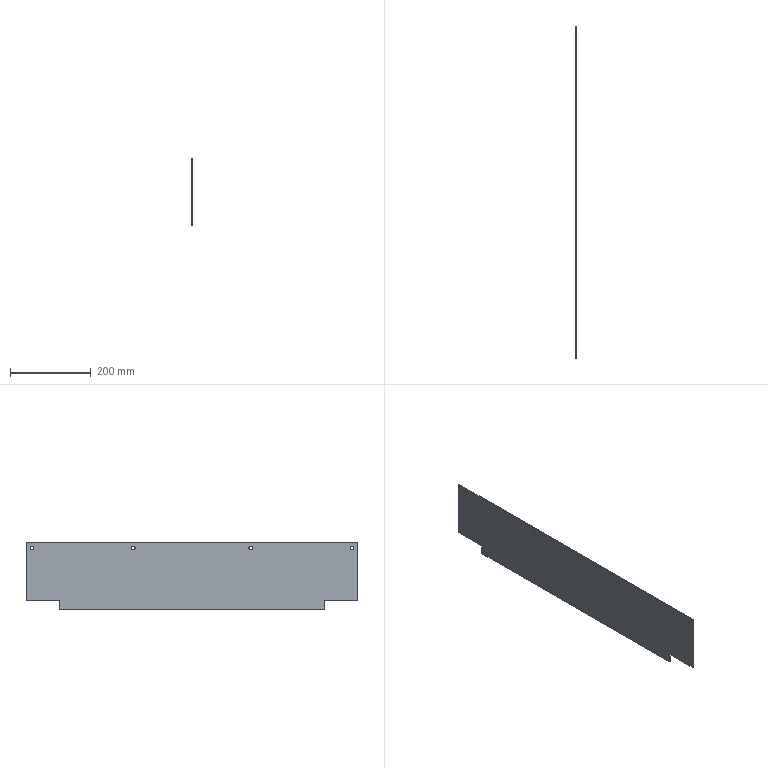Part | STEP file | lll_id2674_x_t | 1 solid | 14 faces | box 2 x 820 x 168 mm | volume 267265 mm3 | plane 10 | cylinder 4 | commonest cylinder face diameters 9 x4
STEP:
#1=CARTESIAN_POINT('',(165.435,-327.7,2.5));
#2=VERTEX_POINT('',#1);
#3=CARTESIAN_POINT('',(165.435,327.5,2.5));
#4=VERTEX_POINT('',#3);
#5=CARTESIAN_POINT('',(165.435,60.,2.5));
#6=DIRECTION('',(0.,1.,0.));
#7=VECTOR('',#6,1.);
#8=LINE('',#5,#7);
#9=EDGE_CURVE('',#2,#4,#8,.T.);
#10=ORIENTED_EDGE('',*,*,#9,.T.);
#11=CARTESIAN_POINT('',(167.435,327.5,2.5));
#12=VERTEX_POINT('',#11);
#13=CARTESIAN_POINT('',(651.435,327.5,2.5));
#14=DIRECTION('',(1.,0.,0.));
#15=VECTOR('',#14,1.);
#16=LINE('',#13,#15);
#17=EDGE_CURVE('',#4,#12,#16,.T.);
#18=ORIENTED_EDGE('',*,*,#17,.T.);
#19=CARTESIAN_POINT('',(167.435,-327.7,2.5));
#20=VERTEX_POINT('',#19);
#21=CARTESIAN_POINT('',(167.435,60.,2.5));
#22=DIRECTION('',(0.,1.,0.));
#23=VECTOR('',#22,1.);
#24=LINE('',#21,#23);
#25=EDGE_CURVE('',#20,#12,#24,.T.);
#26=ORIENTED_EDGE('',*,*,#25,.F.);
#27=CARTESIAN_POINT('',(651.435,-327.7,2.5));
#28=DIRECTION('',(-1.,0.,0.));
#29=VECTOR('',#28,1.);
#30=LINE('',#27,#29);
#31=EDGE_CURVE('',#20,#2,#30,.T.);
#32=ORIENTED_EDGE('',*,*,#31,.T.);
#33=EDGE_LOOP('',(#10,#18,#26,#32));
#34=FACE_OUTER_BOUND('',#33,.T.);
#35=CARTESIAN_POINT('',(651.435,1252.5,2.5));
#36=DIRECTION('',(0.,0.,-1.));
#37=DIRECTION('',(0.,-1.,0.));
#38=AXIS2_PLACEMENT_3D('',#35,#36,#37);
#39=PLANE('',#38);
#40=ADVANCED_FACE('',(#34),#39,.T.);
#41=CARTESIAN_POINT('',(165.435,140.5,155.5));
#42=VERTEX_POINT('',#41);
#43=CARTESIAN_POINT('',(165.435,145.,155.5));
#44=DIRECTION('',(1.,0.,0.));
#45=DIRECTION('',(0.,-1.,0.));
#46=AXIS2_PLACEMENT_3D('',#43,#44,#45);
#47=CIRCLE('',#46,4.5);
#48=EDGE_CURVE('',#42,#42,#47,.T.);
#49=ORIENTED_EDGE('',*,*,#48,.T.);
#50=EDGE_LOOP('',(#49));
#51=FACE_BOUND('',#50,.T.);
#52=CARTESIAN_POINT('',(165.435,399.5,155.5));
#53=VERTEX_POINT('',#52);
#54=CARTESIAN_POINT('',(165.435,395.,155.5));
#55=DIRECTION('',(1.,0.,0.));
#56=DIRECTION('',(0.,1.,0.));
#57=AXIS2_PLACEMENT_3D('',#54,#55,#56);
#58=CIRCLE('',#57,4.5);
#59=EDGE_CURVE('',#53,#53,#58,.T.);
#60=ORIENTED_EDGE('',*,*,#59,.T.);
#61=EDGE_LOOP('',(#60));
#62=FACE_BOUND('',#61,.T.);
#63=CARTESIAN_POINT('',(165.435,-140.5,155.5));
#64=VERTEX_POINT('',#63);
#65=CARTESIAN_POINT('',(165.435,-145.,155.5));
#66=DIRECTION('',(-1.,0.,0.));
#67=DIRECTION('',(0.,1.,0.));
#68=AXIS2_PLACEMENT_3D('',#65,#66,#67);
#69=CIRCLE('',#68,4.5);
#70=EDGE_CURVE('',#64,#64,#69,.T.);
#71=ORIENTED_EDGE('',*,*,#70,.F.);
#72=EDGE_LOOP('',(#71));
#73=FACE_BOUND('',#72,.T.);
#74=CARTESIAN_POINT('',(165.435,-399.5,155.5));
#75=VERTEX_POINT('',#74);
#76=CARTESIAN_POINT('',(165.435,-395.,155.5));
#77=DIRECTION('',(-1.,0.,0.));
#78=DIRECTION('',(0.,-1.,0.));
#79=AXIS2_PLACEMENT_3D('',#76,#77,#78);
#80=CIRCLE('',#79,4.5);
#81=EDGE_CURVE('',#75,#75,#80,.T.);
#82=ORIENTED_EDGE('',*,*,#81,.F.);
#83=EDGE_LOOP('',(#82));
#84=FACE_BOUND('',#83,.T.);
#85=CARTESIAN_POINT('',(165.435,327.5,26.));
#86=VERTEX_POINT('',#85);
#87=CARTESIAN_POINT('',(165.435,327.5,-78.5));
#88=DIRECTION('',(0.,0.,1.));
#89=VECTOR('',#88,1.);
#90=LINE('',#87,#89);
#91=EDGE_CURVE('',#4,#86,#90,.T.);
#92=ORIENTED_EDGE('',*,*,#91,.F.);
#93=ORIENTED_EDGE('',*,*,#9,.F.);
#94=CARTESIAN_POINT('',(165.435,-327.7,26.));
#95=VERTEX_POINT('',#94);
#96=CARTESIAN_POINT('',(165.435,-327.7,-78.5));
#97=DIRECTION('',(0.,0.,-1.));
#98=VECTOR('',#97,1.);
#99=LINE('',#96,#98);
#100=EDGE_CURVE('',#95,#2,#99,.T.);
#101=ORIENTED_EDGE('',*,*,#100,.F.);
#102=CARTESIAN_POINT('',(165.435,-410.,26.));
#103=VERTEX_POINT('',#102);
#104=CARTESIAN_POINT('',(165.435,60.,26.));
#105=DIRECTION('',(0.,1.,0.));
#106=VECTOR('',#105,1.);
#107=LINE('',#104,#106);
#108=EDGE_CURVE('',#103,#95,#107,.T.);
#109=ORIENTED_EDGE('',*,*,#108,.F.);
#110=CARTESIAN_POINT('',(165.435,-410.,170.5));
#111=VERTEX_POINT('',#110);
#112=CARTESIAN_POINT('',(165.435,-410.,-78.5));
#113=DIRECTION('',(0.,0.,-1.));
#114=VECTOR('',#113,1.);
#115=LINE('',#112,#114);
#116=EDGE_CURVE('',#111,#103,#115,.T.);
#117=ORIENTED_EDGE('',*,*,#116,.F.);
#118=CARTESIAN_POINT('',(165.435,410.,170.5));
#119=VERTEX_POINT('',#118);
#120=CARTESIAN_POINT('',(165.435,60.,170.5));
#121=DIRECTION('',(0.,-1.,0.));
#122=VECTOR('',#121,1.);
#123=LINE('',#120,#122);
#124=EDGE_CURVE('',#119,#111,#123,.T.);
#125=ORIENTED_EDGE('',*,*,#124,.F.);
#126=CARTESIAN_POINT('',(165.435,410.,26.));
#127=VERTEX_POINT('',#126);
#128=CARTESIAN_POINT('',(165.435,410.,-78.5));
#129=DIRECTION('',(0.,0.,-1.));
#130=VECTOR('',#129,1.);
#131=LINE('',#128,#130);
#132=EDGE_CURVE('',#119,#127,#131,.T.);
#133=ORIENTED_EDGE('',*,*,#132,.T.);
#134=CARTESIAN_POINT('',(165.435,60.,26.));
#135=DIRECTION('',(0.,1.,0.));
#136=VECTOR('',#135,1.);
#137=LINE('',#134,#136);
#138=EDGE_CURVE('',#86,#127,#137,.T.);
#139=ORIENTED_EDGE('',*,*,#138,.F.);
#140=EDGE_LOOP('',(#92,#93,#101,#109,#117,#125,#133,#139));
#141=FACE_BOUND('',#140,.T.);
#142=CARTESIAN_POINT('',(165.435,60.,-78.5));
#143=DIRECTION('',(1.,0.,0.));
#144=DIRECTION('',(0.,0.,-1.));
#145=AXIS2_PLACEMENT_3D('',#142,#143,#144);
#146=PLANE('',#145);
#147=ADVANCED_FACE('',(#51,#62,#73,#84,#141),#146,.F.);
#148=CARTESIAN_POINT('',(167.435,-390.5,155.5));
#149=VERTEX_POINT('',#148);
#150=CARTESIAN_POINT('',(167.435,-395.,155.5));
#151=DIRECTION('',(-1.,0.,0.));
#152=DIRECTION('',(0.,1.,0.));
#153=AXIS2_PLACEMENT_3D('',#150,#151,#152);
#154=CIRCLE('',#153,4.5);
#155=EDGE_CURVE('',#149,#149,#154,.T.);
#156=ORIENTED_EDGE('',*,*,#155,.T.);
#157=EDGE_LOOP('',(#156));
#158=FACE_BOUND('',#157,.T.);
#159=CARTESIAN_POINT('',(167.435,-140.5,155.5));
#160=VERTEX_POINT('',#159);
#161=CARTESIAN_POINT('',(167.435,-145.,155.5));
#162=DIRECTION('',(-1.,0.,0.));
#163=DIRECTION('',(0.,1.,0.));
#164=AXIS2_PLACEMENT_3D('',#161,#162,#163);
#165=CIRCLE('',#164,4.5);
#166=EDGE_CURVE('',#160,#160,#165,.T.);
#167=ORIENTED_EDGE('',*,*,#166,.T.);
#168=EDGE_LOOP('',(#167));
#169=FACE_BOUND('',#168,.T.);
#170=CARTESIAN_POINT('',(167.435,390.5,155.5));
#171=VERTEX_POINT('',#170);
#172=CARTESIAN_POINT('',(167.435,395.,155.5));
#173=DIRECTION('',(1.,0.,0.));
#174=DIRECTION('',(0.,-1.,0.));
#175=AXIS2_PLACEMENT_3D('',#172,#173,#174);
#176=CIRCLE('',#175,4.5);
#177=EDGE_CURVE('',#171,#171,#176,.T.);
#178=ORIENTED_EDGE('',*,*,#177,.F.);
#179=EDGE_LOOP('',(#178));
#180=FACE_BOUND('',#179,.T.);
#181=CARTESIAN_POINT('',(167.435,140.5,155.5));
#182=VERTEX_POINT('',#181);
#183=CARTESIAN_POINT('',(167.435,145.,155.5));
#184=DIRECTION('',(1.,0.,0.));
#185=DIRECTION('',(0.,-1.,0.));
#186=AXIS2_PLACEMENT_3D('',#183,#184,#185);
#187=CIRCLE('',#186,4.5);
#188=EDGE_CURVE('',#182,#182,#187,.T.);
#189=ORIENTED_EDGE('',*,*,#188,.F.);
#190=EDGE_LOOP('',(#189));
#191=FACE_BOUND('',#190,.T.);
#192=ORIENTED_EDGE('',*,*,#25,.T.);
#193=CARTESIAN_POINT('',(167.435,327.5,26.));
#194=VERTEX_POINT('',#193);
#195=CARTESIAN_POINT('',(167.435,327.5,-78.5));
#196=DIRECTION('',(0.,0.,1.));
#197=VECTOR('',#196,1.);
#198=LINE('',#195,#197);
#199=EDGE_CURVE('',#12,#194,#198,.T.);
#200=ORIENTED_EDGE('',*,*,#199,.T.);
#201=CARTESIAN_POINT('',(167.435,410.,26.));
#202=VERTEX_POINT('',#201);
#203=CARTESIAN_POINT('',(167.435,60.,26.));
#204=DIRECTION('',(0.,1.,0.));
#205=VECTOR('',#204,1.);
#206=LINE('',#203,#205);
#207=EDGE_CURVE('',#194,#202,#206,.T.);
#208=ORIENTED_EDGE('',*,*,#207,.T.);
#209=CARTESIAN_POINT('',(167.435,410.,170.5));
#210=VERTEX_POINT('',#209);
#211=CARTESIAN_POINT('',(167.435,410.,-78.5));
#212=DIRECTION('',(0.,0.,-1.));
#213=VECTOR('',#212,1.);
#214=LINE('',#211,#213);
#215=EDGE_CURVE('',#210,#202,#214,.T.);
#216=ORIENTED_EDGE('',*,*,#215,.F.);
#217=CARTESIAN_POINT('',(167.435,-410.,170.5));
#218=VERTEX_POINT('',#217);
#219=CARTESIAN_POINT('',(167.435,60.,170.5));
#220=DIRECTION('',(0.,-1.,0.));
#221=VECTOR('',#220,1.);
#222=LINE('',#219,#221);
#223=EDGE_CURVE('',#210,#218,#222,.T.);
#224=ORIENTED_EDGE('',*,*,#223,.T.);
#225=CARTESIAN_POINT('',(167.435,-410.,26.));
#226=VERTEX_POINT('',#225);
#227=CARTESIAN_POINT('',(167.435,-410.,-78.5));
#228=DIRECTION('',(0.,0.,-1.));
#229=VECTOR('',#228,1.);
#230=LINE('',#227,#229);
#231=EDGE_CURVE('',#218,#226,#230,.T.);
#232=ORIENTED_EDGE('',*,*,#231,.T.);
#233=CARTESIAN_POINT('',(167.435,-327.7,26.));
#234=VERTEX_POINT('',#233);
#235=CARTESIAN_POINT('',(167.435,60.,26.));
#236=DIRECTION('',(0.,1.,0.));
#237=VECTOR('',#236,1.);
#238=LINE('',#235,#237);
#239=EDGE_CURVE('',#226,#234,#238,.T.);
#240=ORIENTED_EDGE('',*,*,#239,.T.);
#241=CARTESIAN_POINT('',(167.435,-327.7,-78.5));
#242=DIRECTION('',(0.,0.,-1.));
#243=VECTOR('',#242,1.);
#244=LINE('',#241,#243);
#245=EDGE_CURVE('',#234,#20,#244,.T.);
#246=ORIENTED_EDGE('',*,*,#245,.T.);
#247=EDGE_LOOP('',(#192,#200,#208,#216,#224,#232,#240,#246));
#248=FACE_BOUND('',#247,.T.);
#249=CARTESIAN_POINT('',(167.435,60.,-78.5));
#250=DIRECTION('',(1.,0.,0.));
#251=DIRECTION('',(0.,0.,-1.));
#252=AXIS2_PLACEMENT_3D('',#249,#250,#251);
#253=PLANE('',#252);
#254=ADVANCED_FACE('',(#158,#169,#180,#191,#248),#253,.T.);
#255=ORIENTED_EDGE('',*,*,#207,.F.);
#256=CARTESIAN_POINT('',(217.435,327.5,26.));
#257=DIRECTION('',(-1.,0.,0.));
#258=VECTOR('',#257,1.);
#259=LINE('',#256,#258);
#260=EDGE_CURVE('',#194,#86,#259,.T.);
#261=ORIENTED_EDGE('',*,*,#260,.T.);
#262=ORIENTED_EDGE('',*,*,#138,.T.);
#263=CARTESIAN_POINT('',(217.435,410.,26.));
#264=DIRECTION('',(1.,0.,0.));
#265=VECTOR('',#264,1.);
#266=LINE('',#263,#265);
#267=EDGE_CURVE('',#127,#202,#266,.T.);
#268=ORIENTED_EDGE('',*,*,#267,.T.);
#269=EDGE_LOOP('',(#255,#261,#262,#268));
#270=FACE_OUTER_BOUND('',#269,.T.);
#271=CARTESIAN_POINT('',(217.435,367.5,26.));
#272=DIRECTION('',(0.,0.,1.));
#273=DIRECTION('',(1.,0.,0.));
#274=AXIS2_PLACEMENT_3D('',#271,#272,#273);
#275=PLANE('',#274);
#276=ADVANCED_FACE('',(#270),#275,.F.);
#277=ORIENTED_EDGE('',*,*,#108,.T.);
#278=CARTESIAN_POINT('',(227.435,-327.7,26.));
#279=DIRECTION('',(1.,0.,0.));
#280=VECTOR('',#279,1.);
#281=LINE('',#278,#280);
#282=EDGE_CURVE('',#95,#234,#281,.T.);
#283=ORIENTED_EDGE('',*,*,#282,.T.);
#284=ORIENTED_EDGE('',*,*,#239,.F.);
#285=CARTESIAN_POINT('',(165.435,-410.,26.));
#286=DIRECTION('',(1.,0.,0.));
#287=VECTOR('',#286,1.);
#288=LINE('',#285,#287);
#289=EDGE_CURVE('',#103,#226,#288,.T.);
#290=ORIENTED_EDGE('',*,*,#289,.F.);
#291=EDGE_LOOP('',(#277,#283,#284,#290));
#292=FACE_OUTER_BOUND('',#291,.T.);
#293=CARTESIAN_POINT('',(227.435,-370.7,26.));
#294=DIRECTION('',(0.,0.,1.));
#295=DIRECTION('',(-1.,0.,0.));
#296=AXIS2_PLACEMENT_3D('',#293,#294,#295);
#297=PLANE('',#296);
#298=ADVANCED_FACE('',(#292),#297,.F.);
#299=ORIENTED_EDGE('',*,*,#231,.F.);
#300=CARTESIAN_POINT('',(167.435,-410.,170.5));
#301=DIRECTION('',(-1.,0.,0.));
#302=VECTOR('',#301,1.);
#303=LINE('',#300,#302);
#304=EDGE_CURVE('',#218,#111,#303,.T.);
#305=ORIENTED_EDGE('',*,*,#304,.T.);
#306=ORIENTED_EDGE('',*,*,#116,.T.);
#307=ORIENTED_EDGE('',*,*,#289,.T.);
#308=EDGE_LOOP('',(#299,#305,#306,#307));
#309=FACE_OUTER_BOUND('',#308,.T.);
#310=CARTESIAN_POINT('',(165.435,-410.,-78.5));
#311=DIRECTION('',(0.,1.,0.));
#312=DIRECTION('',(0.,0.,-1.));
#313=AXIS2_PLACEMENT_3D('',#310,#311,#312);
#314=PLANE('',#313);
#315=ADVANCED_FACE('',(#309),#314,.F.);
#316=CARTESIAN_POINT('',(167.435,410.,170.5));
#317=DIRECTION('',(-1.,0.,0.));
#318=VECTOR('',#317,1.);
#319=LINE('',#316,#318);
#320=EDGE_CURVE('',#210,#119,#319,.T.);
#321=ORIENTED_EDGE('',*,*,#320,.F.);
#322=ORIENTED_EDGE('',*,*,#215,.T.);
#323=ORIENTED_EDGE('',*,*,#267,.F.);
#324=ORIENTED_EDGE('',*,*,#132,.F.);
#325=EDGE_LOOP('',(#321,#322,#323,#324));
#326=FACE_OUTER_BOUND('',#325,.T.);
#327=CARTESIAN_POINT('',(165.435,410.,-78.5));
#328=DIRECTION('',(0.,-1.,0.));
#329=DIRECTION('',(0.,0.,-1.));
#330=AXIS2_PLACEMENT_3D('',#327,#328,#329);
#331=PLANE('',#330);
#332=ADVANCED_FACE('',(#326),#331,.F.);
#333=ORIENTED_EDGE('',*,*,#124,.T.);
#334=ORIENTED_EDGE('',*,*,#304,.F.);
#335=ORIENTED_EDGE('',*,*,#223,.F.);
#336=ORIENTED_EDGE('',*,*,#320,.T.);
#337=EDGE_LOOP('',(#333,#334,#335,#336));
#338=FACE_OUTER_BOUND('',#337,.T.);
#339=CARTESIAN_POINT('',(167.435,60.,170.5));
#340=DIRECTION('',(0.,0.,1.));
#341=DIRECTION('',(0.,1.,0.));
#342=AXIS2_PLACEMENT_3D('',#339,#340,#341);
#343=PLANE('',#342);
#344=ADVANCED_FACE('',(#338),#343,.T.);
#345=ORIENTED_EDGE('',*,*,#177,.T.);
#346=EDGE_LOOP('',(#345));
#347=FACE_BOUND('',#346,.T.);
#348=ORIENTED_EDGE('',*,*,#59,.F.);
#349=EDGE_LOOP('',(#348));
#350=FACE_BOUND('',#349,.T.);
#351=CARTESIAN_POINT('',(165.435,395.,155.5));
#352=DIRECTION('',(1.,0.,0.));
#353=DIRECTION('',(0.,1.,0.));
#354=AXIS2_PLACEMENT_3D('',#351,#352,#353);
#355=CYLINDRICAL_SURFACE('',#354,4.5);
#356=ADVANCED_FACE('',(#347,#350),#355,.F.);
#357=ORIENTED_EDGE('',*,*,#188,.T.);
#358=EDGE_LOOP('',(#357));
#359=FACE_BOUND('',#358,.T.);
#360=ORIENTED_EDGE('',*,*,#48,.F.);
#361=EDGE_LOOP('',(#360));
#362=FACE_BOUND('',#361,.T.);
#363=CARTESIAN_POINT('',(165.435,145.,155.5));
#364=DIRECTION('',(1.,0.,0.));
#365=DIRECTION('',(0.,-1.,0.));
#366=AXIS2_PLACEMENT_3D('',#363,#364,#365);
#367=CYLINDRICAL_SURFACE('',#366,4.5);
#368=ADVANCED_FACE('',(#359,#362),#367,.F.);
#369=ORIENTED_EDGE('',*,*,#155,.F.);
#370=EDGE_LOOP('',(#369));
#371=FACE_BOUND('',#370,.T.);
#372=ORIENTED_EDGE('',*,*,#81,.T.);
#373=EDGE_LOOP('',(#372));
#374=FACE_BOUND('',#373,.T.);
#375=CARTESIAN_POINT('',(165.435,-395.,155.5));
#376=DIRECTION('',(1.,0.,0.));
#377=DIRECTION('',(0.,-1.,0.));
#378=AXIS2_PLACEMENT_3D('',#375,#376,#377);
#379=CYLINDRICAL_SURFACE('',#378,4.5);
#380=ADVANCED_FACE('',(#371,#374),#379,.F.);
#381=ORIENTED_EDGE('',*,*,#166,.F.);
#382=EDGE_LOOP('',(#381));
#383=FACE_BOUND('',#382,.T.);
#384=ORIENTED_EDGE('',*,*,#70,.T.);
#385=EDGE_LOOP('',(#384));
#386=FACE_BOUND('',#385,.T.);
#387=CARTESIAN_POINT('',(165.435,-145.,155.5));
#388=DIRECTION('',(1.,0.,0.));
#389=DIRECTION('',(0.,1.,0.));
#390=AXIS2_PLACEMENT_3D('',#387,#388,#389);
#391=CYLINDRICAL_SURFACE('',#390,4.5);
#392=ADVANCED_FACE('',(#383,#386),#391,.F.);
#393=ORIENTED_EDGE('',*,*,#100,.T.);
#394=ORIENTED_EDGE('',*,*,#31,.F.);
#395=ORIENTED_EDGE('',*,*,#245,.F.);
#396=ORIENTED_EDGE('',*,*,#282,.F.);
#397=EDGE_LOOP('',(#393,#394,#395,#396));
#398=FACE_OUTER_BOUND('',#397,.T.);
#399=CARTESIAN_POINT('',(227.435,-327.7,16.));
#400=DIRECTION('',(0.,-1.,0.));
#401=DIRECTION('',(0.,0.,1.));
#402=AXIS2_PLACEMENT_3D('',#399,#400,#401);
#403=PLANE('',#402);
#404=ADVANCED_FACE('',(#398),#403,.T.);
#405=ORIENTED_EDGE('',*,*,#91,.T.);
#406=ORIENTED_EDGE('',*,*,#260,.F.);
#407=ORIENTED_EDGE('',*,*,#199,.F.);
#408=ORIENTED_EDGE('',*,*,#17,.F.);
#409=EDGE_LOOP('',(#405,#406,#407,#408));
#410=FACE_OUTER_BOUND('',#409,.T.);
#411=CARTESIAN_POINT('',(217.435,327.5,16.));
#412=DIRECTION('',(0.,1.,0.));
#413=DIRECTION('',(0.,0.,1.));
#414=AXIS2_PLACEMENT_3D('',#411,#412,#413);
#415=PLANE('',#414);
#416=ADVANCED_FACE('',(#410),#415,.T.);
#417=CLOSED_SHELL('',(#40,#147,#254,#276,#298,#315,#332,#344,#356,#368,#380,#392,#404,#416));
#418=MANIFOLD_SOLID_BREP('',#417);
#419=(LENGTH_UNIT()NAMED_UNIT(*)SI_UNIT(.MILLI.,.METRE.));
#420=UNCERTAINTY_MEASURE_WITH_UNIT(LENGTH_MEASURE(0.00002),#419,'','');
#421=(NAMED_UNIT(*)PLANE_ANGLE_UNIT()SI_UNIT($,.RADIAN.));
#422=PLANE_ANGLE_MEASURE_WITH_UNIT(PLANE_ANGLE_MEASURE(0.01745),#421);
#423=DIMENSIONAL_EXPONENTS(0.,0.,0.,0.,0.,0.,0.);
#424=(CONVERSION_BASED_UNIT('DEGREE',#422)NAMED_UNIT(#423)PLANE_ANGLE_UNIT());
#425=(NAMED_UNIT(*)SI_UNIT($,.STERADIAN.)SOLID_ANGLE_UNIT());
#426=(GEOMETRIC_REPRESENTATION_CONTEXT(3)GLOBAL_UNCERTAINTY_ASSIGNED_CONTEXT((#420))GLOBAL_UNIT_ASSIGNED_CONTEXT((#419,#424,#425))REPRESENTATION_CONTEXT('',''));
#427=ADVANCED_BREP_SHAPE_REPRESENTATION('',(#418),#426);